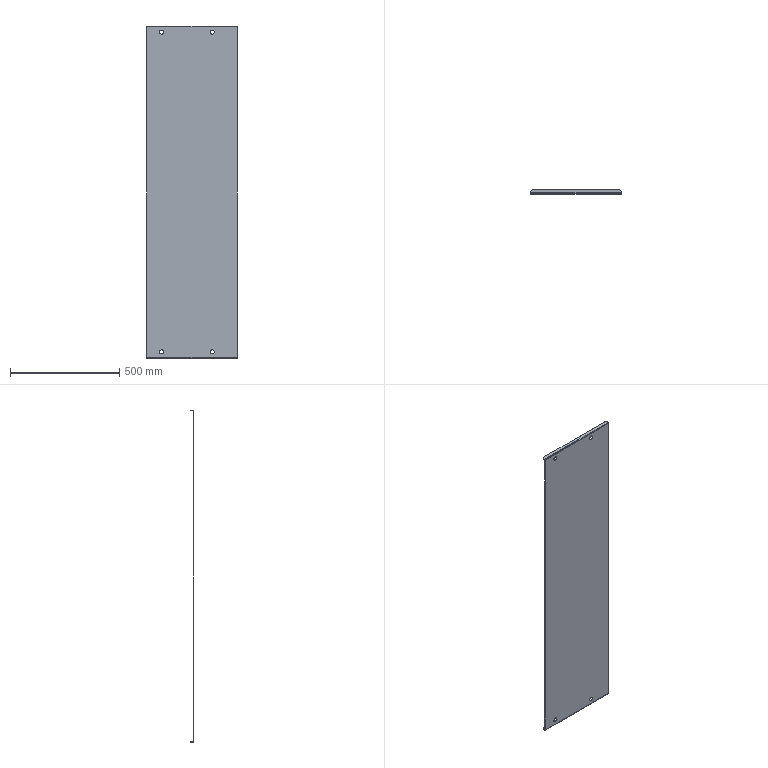Part | SolidWorks | features Fillet 1, FlatPattern 1, ICE 1, SMBaseFlange 1, SheetMetal 1 | 1 solid | 34 faces | box 413 x 18 x 1520 mm | volume 1023020 mm3 | plane 18 | cylinder 16 | commonest cylinder face diameters 18 x8 20 x4 3 x2 6.2 x2
STEP:
#1=CARTESIAN_POINT('',(-139.5,1.6,-1483.));
#2=VERTEX_POINT('',#1);
#3=CARTESIAN_POINT('',(-139.5,1.6,-1501.));
#4=VERTEX_POINT('',#3);
#5=CARTESIAN_POINT('',(-139.5,1.6,-1492.));
#6=DIRECTION('',(0.,-1.,0.));
#7=DIRECTION('',(0.,0.,1.));
#8=AXIS2_PLACEMENT_3D('',#5,#6,#7);
#9=CIRCLE('',#8,9.);
#10=EDGE_CURVE('',#2,#4,#9,.T.);
#11=ORIENTED_EDGE('',*,*,#10,.F.);
#12=CARTESIAN_POINT('',(-139.5,0.,-1483.));
#13=VERTEX_POINT('',#12);
#14=CARTESIAN_POINT('',(-139.5,18.001,-1483.));
#15=DIRECTION('',(0.,-1.,0.));
#16=VECTOR('',#15,1000.);
#17=LINE('',#14,#16);
#18=EDGE_CURVE('',#2,#13,#17,.T.);
#19=ORIENTED_EDGE('',*,*,#18,.T.);
#20=CARTESIAN_POINT('',(-139.5,0.,-1501.));
#21=VERTEX_POINT('',#20);
#22=CARTESIAN_POINT('',(-139.5,0.,-1492.));
#23=DIRECTION('',(0.,-1.,0.));
#24=DIRECTION('',(0.,0.,1.));
#25=AXIS2_PLACEMENT_3D('',#22,#23,#24);
#26=CIRCLE('',#25,9.);
#27=EDGE_CURVE('',#13,#21,#26,.T.);
#28=ORIENTED_EDGE('',*,*,#27,.T.);
#29=CARTESIAN_POINT('',(-139.5,18.001,-1501.));
#30=DIRECTION('',(0.,-1.,0.));
#31=VECTOR('',#30,1000.);
#32=LINE('',#29,#31);
#33=EDGE_CURVE('',#4,#21,#32,.T.);
#34=ORIENTED_EDGE('',*,*,#33,.F.);
#35=EDGE_LOOP('',(#11,#19,#28,#34));
#36=FACE_OUTER_BOUND('',#35,.T.);
#37=CARTESIAN_POINT('',(-139.5,18.001,-1492.));
#38=DIRECTION('',(0.,-1.,0.));
#39=DIRECTION('',(0.,0.,-1.));
#40=AXIS2_PLACEMENT_3D('',#37,#38,#39);
#41=CYLINDRICAL_SURFACE('',#40,9.);
#42=ADVANCED_FACE('',(#36),#41,.F.);
#43=CARTESIAN_POINT('',(92.5,1.6,-1483.));
#44=VERTEX_POINT('',#43);
#45=CARTESIAN_POINT('',(92.5,1.6,-1501.));
#46=VERTEX_POINT('',#45);
#47=CARTESIAN_POINT('',(92.5,1.6,-1492.));
#48=DIRECTION('',(0.,-1.,0.));
#49=DIRECTION('',(0.,0.,1.));
#50=AXIS2_PLACEMENT_3D('',#47,#48,#49);
#51=CIRCLE('',#50,9.);
#52=EDGE_CURVE('',#44,#46,#51,.T.);
#53=ORIENTED_EDGE('',*,*,#52,.F.);
#54=CARTESIAN_POINT('',(92.5,0.,-1483.));
#55=VERTEX_POINT('',#54);
#56=CARTESIAN_POINT('',(92.5,18.001,-1483.));
#57=DIRECTION('',(0.,-1.,0.));
#58=VECTOR('',#57,1000.);
#59=LINE('',#56,#58);
#60=EDGE_CURVE('',#44,#55,#59,.T.);
#61=ORIENTED_EDGE('',*,*,#60,.T.);
#62=CARTESIAN_POINT('',(92.5,0.,-1501.));
#63=VERTEX_POINT('',#62);
#64=CARTESIAN_POINT('',(92.5,0.,-1492.));
#65=DIRECTION('',(0.,-1.,0.));
#66=DIRECTION('',(0.,0.,1.));
#67=AXIS2_PLACEMENT_3D('',#64,#65,#66);
#68=CIRCLE('',#67,9.);
#69=EDGE_CURVE('',#55,#63,#68,.T.);
#70=ORIENTED_EDGE('',*,*,#69,.T.);
#71=CARTESIAN_POINT('',(92.5,18.001,-1501.));
#72=DIRECTION('',(0.,-1.,0.));
#73=VECTOR('',#72,1000.);
#74=LINE('',#71,#73);
#75=EDGE_CURVE('',#46,#63,#74,.T.);
#76=ORIENTED_EDGE('',*,*,#75,.F.);
#77=EDGE_LOOP('',(#53,#61,#70,#76));
#78=FACE_OUTER_BOUND('',#77,.T.);
#79=CARTESIAN_POINT('',(92.5,18.001,-1492.));
#80=DIRECTION('',(0.,-1.,0.));
#81=DIRECTION('',(0.,0.,-1.));
#82=AXIS2_PLACEMENT_3D('',#79,#80,#81);
#83=CYLINDRICAL_SURFACE('',#82,9.);
#84=ADVANCED_FACE('',(#78),#83,.F.);
#85=CARTESIAN_POINT('',(92.5,1.6,-19.));
#86=VERTEX_POINT('',#85);
#87=CARTESIAN_POINT('',(92.5,1.6,-37.));
#88=VERTEX_POINT('',#87);
#89=CARTESIAN_POINT('',(92.5,1.6,-28.));
#90=DIRECTION('',(0.,-1.,0.));
#91=DIRECTION('',(0.,0.,1.));
#92=AXIS2_PLACEMENT_3D('',#89,#90,#91);
#93=CIRCLE('',#92,9.);
#94=EDGE_CURVE('',#86,#88,#93,.T.);
#95=ORIENTED_EDGE('',*,*,#94,.F.);
#96=CARTESIAN_POINT('',(92.5,0.,-19.));
#97=VERTEX_POINT('',#96);
#98=CARTESIAN_POINT('',(92.5,18.001,-19.));
#99=DIRECTION('',(0.,-1.,0.));
#100=VECTOR('',#99,1000.);
#101=LINE('',#98,#100);
#102=EDGE_CURVE('',#86,#97,#101,.T.);
#103=ORIENTED_EDGE('',*,*,#102,.T.);
#104=CARTESIAN_POINT('',(92.5,0.,-37.));
#105=VERTEX_POINT('',#104);
#106=CARTESIAN_POINT('',(92.5,0.,-28.));
#107=DIRECTION('',(0.,-1.,0.));
#108=DIRECTION('',(0.,0.,-1.));
#109=AXIS2_PLACEMENT_3D('',#106,#107,#108);
#110=CIRCLE('',#109,9.);
#111=EDGE_CURVE('',#97,#105,#110,.T.);
#112=ORIENTED_EDGE('',*,*,#111,.T.);
#113=CARTESIAN_POINT('',(92.5,18.001,-37.));
#114=DIRECTION('',(0.,-1.,0.));
#115=VECTOR('',#114,1000.);
#116=LINE('',#113,#115);
#117=EDGE_CURVE('',#88,#105,#116,.T.);
#118=ORIENTED_EDGE('',*,*,#117,.F.);
#119=EDGE_LOOP('',(#95,#103,#112,#118));
#120=FACE_OUTER_BOUND('',#119,.T.);
#121=CARTESIAN_POINT('',(92.5,18.001,-28.));
#122=DIRECTION('',(0.,-1.,0.));
#123=DIRECTION('',(0.,0.,-1.));
#124=AXIS2_PLACEMENT_3D('',#121,#122,#123);
#125=CYLINDRICAL_SURFACE('',#124,9.);
#126=ADVANCED_FACE('',(#120),#125,.F.);
#127=CARTESIAN_POINT('',(-139.5,1.6,-19.));
#128=VERTEX_POINT('',#127);
#129=CARTESIAN_POINT('',(-139.5,1.6,-37.));
#130=VERTEX_POINT('',#129);
#131=CARTESIAN_POINT('',(-139.5,1.6,-28.));
#132=DIRECTION('',(0.,-1.,0.));
#133=DIRECTION('',(0.,0.,1.));
#134=AXIS2_PLACEMENT_3D('',#131,#132,#133);
#135=CIRCLE('',#134,9.);
#136=EDGE_CURVE('',#128,#130,#135,.T.);
#137=ORIENTED_EDGE('',*,*,#136,.F.);
#138=CARTESIAN_POINT('',(-139.5,0.,-19.));
#139=VERTEX_POINT('',#138);
#140=CARTESIAN_POINT('',(-139.5,18.001,-19.));
#141=DIRECTION('',(0.,-1.,0.));
#142=VECTOR('',#141,1000.);
#143=LINE('',#140,#142);
#144=EDGE_CURVE('',#128,#139,#143,.T.);
#145=ORIENTED_EDGE('',*,*,#144,.T.);
#146=CARTESIAN_POINT('',(-139.5,0.,-37.));
#147=VERTEX_POINT('',#146);
#148=CARTESIAN_POINT('',(-139.5,0.,-28.));
#149=DIRECTION('',(0.,-1.,0.));
#150=DIRECTION('',(0.,0.,-1.));
#151=AXIS2_PLACEMENT_3D('',#148,#149,#150);
#152=CIRCLE('',#151,9.);
#153=EDGE_CURVE('',#139,#147,#152,.T.);
#154=ORIENTED_EDGE('',*,*,#153,.T.);
#155=CARTESIAN_POINT('',(-139.5,18.001,-37.));
#156=DIRECTION('',(0.,-1.,0.));
#157=VECTOR('',#156,1000.);
#158=LINE('',#155,#157);
#159=EDGE_CURVE('',#130,#147,#158,.T.);
#160=ORIENTED_EDGE('',*,*,#159,.F.);
#161=EDGE_LOOP('',(#137,#145,#154,#160));
#162=FACE_OUTER_BOUND('',#161,.T.);
#163=CARTESIAN_POINT('',(-139.5,18.001,-28.));
#164=DIRECTION('',(0.,-1.,0.));
#165=DIRECTION('',(0.,0.,-1.));
#166=AXIS2_PLACEMENT_3D('',#163,#164,#165);
#167=CYLINDRICAL_SURFACE('',#166,9.);
#168=ADVANCED_FACE('',(#162),#167,.F.);
#169=CARTESIAN_POINT('',(206.5,3.1,0.));
#170=VERTEX_POINT('',#169);
#171=CARTESIAN_POINT('',(206.5,3.1,-1.6));
#172=VERTEX_POINT('',#171);
#173=CARTESIAN_POINT('',(206.5,3.1,0.));
#174=DIRECTION('',(0.,0.,-1.));
#175=VECTOR('',#174,1000.);
#176=LINE('',#173,#175);
#177=EDGE_CURVE('',#170,#172,#176,.T.);
#178=ORIENTED_EDGE('',*,*,#177,.F.);
#179=CARTESIAN_POINT('',(206.5,0.,-3.1));
#180=VERTEX_POINT('',#179);
#181=CARTESIAN_POINT('',(206.5,3.1,-3.1));
#182=DIRECTION('',(1.,0.,0.));
#183=DIRECTION('',(0.,0.,1.));
#184=AXIS2_PLACEMENT_3D('',#181,#182,#183);
#185=CIRCLE('',#184,3.1);
#186=EDGE_CURVE('',#170,#180,#185,.T.);
#187=ORIENTED_EDGE('',*,*,#186,.T.);
#188=CARTESIAN_POINT('',(206.5,1.6,-3.1));
#189=VERTEX_POINT('',#188);
#190=CARTESIAN_POINT('',(206.5,1.6,-3.1));
#191=DIRECTION('',(0.,-1.,0.));
#192=VECTOR('',#191,1000.);
#193=LINE('',#190,#192);
#194=EDGE_CURVE('',#189,#180,#193,.T.);
#195=ORIENTED_EDGE('',*,*,#194,.F.);
#196=CARTESIAN_POINT('',(206.5,3.1,-3.1));
#197=DIRECTION('',(1.,0.,0.));
#198=DIRECTION('',(0.,0.,-1.));
#199=AXIS2_PLACEMENT_3D('',#196,#197,#198);
#200=CIRCLE('',#199,1.5);
#201=EDGE_CURVE('',#172,#189,#200,.T.);
#202=ORIENTED_EDGE('',*,*,#201,.F.);
#203=EDGE_LOOP('',(#178,#187,#195,#202));
#204=FACE_OUTER_BOUND('',#203,.T.);
#205=CARTESIAN_POINT('',(206.5,3.1,0.));
#206=DIRECTION('',(1.,0.,0.));
#207=DIRECTION('',(0.,0.,-1.));
#208=AXIS2_PLACEMENT_3D('',#205,#206,#207);
#209=PLANE('',#208);
#210=ADVANCED_FACE('',(#204),#209,.T.);
#211=CARTESIAN_POINT('',(206.5,8.,-1.6));
#212=VERTEX_POINT('',#211);
#213=CARTESIAN_POINT('',(206.5,0.,-1.6));
#214=DIRECTION('',(0.,-1.,0.));
#215=VECTOR('',#214,1000.);
#216=LINE('',#213,#215);
#217=EDGE_CURVE('',#212,#172,#216,.T.);
#218=ORIENTED_EDGE('',*,*,#217,.F.);
#219=CARTESIAN_POINT('',(206.5,8.,0.));
#220=VERTEX_POINT('',#219);
#221=CARTESIAN_POINT('',(206.5,8.,-3.1));
#222=DIRECTION('',(0.,0.,1.));
#223=VECTOR('',#222,1000.);
#224=LINE('',#221,#223);
#225=EDGE_CURVE('',#212,#220,#224,.T.);
#226=ORIENTED_EDGE('',*,*,#225,.T.);
#227=CARTESIAN_POINT('',(206.5,0.,0.));
#228=DIRECTION('',(0.,-1.,0.));
#229=VECTOR('',#228,1000.);
#230=LINE('',#227,#229);
#231=EDGE_CURVE('',#220,#170,#230,.T.);
#232=ORIENTED_EDGE('',*,*,#231,.T.);
#233=ORIENTED_EDGE('',*,*,#177,.T.);
#234=EDGE_LOOP('',(#218,#226,#232,#233));
#235=FACE_OUTER_BOUND('',#234,.T.);
#236=CARTESIAN_POINT('',(206.5,1.6,-3.1));
#237=DIRECTION('',(1.,0.,0.));
#238=DIRECTION('',(0.,0.,-1.));
#239=AXIS2_PLACEMENT_3D('',#236,#237,#238);
#240=PLANE('',#239);
#241=ADVANCED_FACE('',(#235),#240,.T.);
#242=CARTESIAN_POINT('',(-206.5,0.,-3.1));
#243=VERTEX_POINT('',#242);
#244=CARTESIAN_POINT('',(-206.5,1.6,-3.1));
#245=VERTEX_POINT('',#244);
#246=CARTESIAN_POINT('',(-206.5,0.,-3.1));
#247=DIRECTION('',(0.,1.,0.));
#248=VECTOR('',#247,1000.);
#249=LINE('',#246,#248);
#250=EDGE_CURVE('',#243,#245,#249,.T.);
#251=ORIENTED_EDGE('',*,*,#250,.F.);
#252=CARTESIAN_POINT('',(-206.5,3.1,0.));
#253=VERTEX_POINT('',#252);
#254=CARTESIAN_POINT('',(-206.5,3.1,-3.1));
#255=DIRECTION('',(1.,0.,0.));
#256=DIRECTION('',(0.,0.,1.));
#257=AXIS2_PLACEMENT_3D('',#254,#255,#256);
#258=CIRCLE('',#257,3.1);
#259=EDGE_CURVE('',#253,#243,#258,.T.);
#260=ORIENTED_EDGE('',*,*,#259,.F.);
#261=CARTESIAN_POINT('',(-206.5,3.1,-1.6));
#262=VERTEX_POINT('',#261);
#263=CARTESIAN_POINT('',(-206.5,3.1,-1.6));
#264=DIRECTION('',(0.,0.,1.));
#265=VECTOR('',#264,1000.);
#266=LINE('',#263,#265);
#267=EDGE_CURVE('',#262,#253,#266,.T.);
#268=ORIENTED_EDGE('',*,*,#267,.F.);
#269=CARTESIAN_POINT('',(-206.5,3.1,-3.1));
#270=DIRECTION('',(1.,0.,0.));
#271=DIRECTION('',(0.,0.,-1.));
#272=AXIS2_PLACEMENT_3D('',#269,#270,#271);
#273=CIRCLE('',#272,1.5);
#274=EDGE_CURVE('',#262,#245,#273,.T.);
#275=ORIENTED_EDGE('',*,*,#274,.T.);
#276=EDGE_LOOP('',(#251,#260,#268,#275));
#277=FACE_OUTER_BOUND('',#276,.T.);
#278=CARTESIAN_POINT('',(-206.5,0.,-3.1));
#279=DIRECTION('',(-1.,0.,0.));
#280=DIRECTION('',(0.,0.,1.));
#281=AXIS2_PLACEMENT_3D('',#278,#279,#280);
#282=PLANE('',#281);
#283=ADVANCED_FACE('',(#277),#282,.T.);
#284=CARTESIAN_POINT('',(-206.5,0.,-1516.9));
#285=VERTEX_POINT('',#284);
#286=CARTESIAN_POINT('',(-206.5,0.,0.));
#287=DIRECTION('',(0.,0.,-1.));
#288=VECTOR('',#287,1000.);
#289=LINE('',#286,#288);
#290=EDGE_CURVE('',#243,#285,#289,.T.);
#291=ORIENTED_EDGE('',*,*,#290,.F.);
#292=ORIENTED_EDGE('',*,*,#250,.T.);
#293=CARTESIAN_POINT('',(-206.5,1.6,-1516.9));
#294=VERTEX_POINT('',#293);
#295=CARTESIAN_POINT('',(-206.5,1.6,0.));
#296=DIRECTION('',(0.,0.,-1.));
#297=VECTOR('',#296,1000.);
#298=LINE('',#295,#297);
#299=EDGE_CURVE('',#245,#294,#298,.T.);
#300=ORIENTED_EDGE('',*,*,#299,.T.);
#301=CARTESIAN_POINT('',(-206.5,1.6,-1516.9));
#302=DIRECTION('',(0.,-1.,0.));
#303=VECTOR('',#302,1000.);
#304=LINE('',#301,#303);
#305=EDGE_CURVE('',#294,#285,#304,.T.);
#306=ORIENTED_EDGE('',*,*,#305,.T.);
#307=EDGE_LOOP('',(#291,#292,#300,#306));
#308=FACE_OUTER_BOUND('',#307,.T.);
#309=CARTESIAN_POINT('',(-206.5,3.1,-1.6));
#310=DIRECTION('',(-1.,0.,0.));
#311=DIRECTION('',(0.,0.,1.));
#312=AXIS2_PLACEMENT_3D('',#309,#310,#311);
#313=PLANE('',#312);
#314=ADVANCED_FACE('',(#308),#313,.T.);
#315=CARTESIAN_POINT('',(206.5,0.,-1516.9));
#316=VERTEX_POINT('',#315);
#317=CARTESIAN_POINT('',(206.5,1.6,-1516.9));
#318=VERTEX_POINT('',#317);
#319=CARTESIAN_POINT('',(206.5,0.,-1516.9));
#320=DIRECTION('',(0.,1.,0.));
#321=VECTOR('',#320,1000.);
#322=LINE('',#319,#321);
#323=EDGE_CURVE('',#316,#318,#322,.T.);
#324=ORIENTED_EDGE('',*,*,#323,.F.);
#325=CARTESIAN_POINT('',(206.5,3.1,-1520.));
#326=VERTEX_POINT('',#325);
#327=CARTESIAN_POINT('',(206.5,3.1,-1516.9));
#328=DIRECTION('',(1.,0.,0.));
#329=DIRECTION('',(0.,0.,1.));
#330=AXIS2_PLACEMENT_3D('',#327,#328,#329);
#331=CIRCLE('',#330,3.1);
#332=EDGE_CURVE('',#316,#326,#331,.T.);
#333=ORIENTED_EDGE('',*,*,#332,.T.);
#334=CARTESIAN_POINT('',(206.5,3.1,-1518.4));
#335=VERTEX_POINT('',#334);
#336=CARTESIAN_POINT('',(206.5,3.1,-1518.4));
#337=DIRECTION('',(0.,0.,-1.));
#338=VECTOR('',#337,1000.);
#339=LINE('',#336,#338);
#340=EDGE_CURVE('',#335,#326,#339,.T.);
#341=ORIENTED_EDGE('',*,*,#340,.F.);
#342=CARTESIAN_POINT('',(206.5,3.1,-1516.9));
#343=DIRECTION('',(1.,0.,0.));
#344=DIRECTION('',(0.,0.,-1.));
#345=AXIS2_PLACEMENT_3D('',#342,#343,#344);
#346=CIRCLE('',#345,1.5);
#347=EDGE_CURVE('',#318,#335,#346,.T.);
#348=ORIENTED_EDGE('',*,*,#347,.F.);
#349=EDGE_LOOP('',(#324,#333,#341,#348));
#350=FACE_OUTER_BOUND('',#349,.T.);
#351=CARTESIAN_POINT('',(206.5,0.,-1516.9));
#352=DIRECTION('',(1.,0.,0.));
#353=DIRECTION('',(0.,0.,-1.));
#354=AXIS2_PLACEMENT_3D('',#351,#352,#353);
#355=PLANE('',#354);
#356=ADVANCED_FACE('',(#350),#355,.T.);
#357=CARTESIAN_POINT('',(206.5,0.,0.));
#358=DIRECTION('',(0.,0.,-1.));
#359=VECTOR('',#358,1000.);
#360=LINE('',#357,#359);
#361=EDGE_CURVE('',#180,#316,#360,.T.);
#362=ORIENTED_EDGE('',*,*,#361,.T.);
#363=ORIENTED_EDGE('',*,*,#323,.T.);
#364=CARTESIAN_POINT('',(206.5,1.6,0.));
#365=DIRECTION('',(0.,0.,-1.));
#366=VECTOR('',#365,1000.);
#367=LINE('',#364,#366);
#368=EDGE_CURVE('',#189,#318,#367,.T.);
#369=ORIENTED_EDGE('',*,*,#368,.F.);
#370=ORIENTED_EDGE('',*,*,#194,.T.);
#371=EDGE_LOOP('',(#362,#363,#369,#370));
#372=FACE_OUTER_BOUND('',#371,.T.);
#373=CARTESIAN_POINT('',(206.5,3.1,-1518.4));
#374=DIRECTION('',(1.,0.,0.));
#375=DIRECTION('',(0.,0.,-1.));
#376=AXIS2_PLACEMENT_3D('',#373,#374,#375);
#377=PLANE('',#376);
#378=ADVANCED_FACE('',(#372),#377,.T.);
#379=CARTESIAN_POINT('',(-206.5,3.1,-1520.));
#380=VERTEX_POINT('',#379);
#381=CARTESIAN_POINT('',(-206.5,3.1,-1518.4));
#382=VERTEX_POINT('',#381);
#383=CARTESIAN_POINT('',(-206.5,3.1,-1520.));
#384=DIRECTION('',(0.,0.,1.));
#385=VECTOR('',#384,1000.);
#386=LINE('',#383,#385);
#387=EDGE_CURVE('',#380,#382,#386,.T.);
#388=ORIENTED_EDGE('',*,*,#387,.F.);
#389=CARTESIAN_POINT('',(-206.5,3.1,-1516.9));
#390=DIRECTION('',(1.,0.,0.));
#391=DIRECTION('',(0.,0.,1.));
#392=AXIS2_PLACEMENT_3D('',#389,#390,#391);
#393=CIRCLE('',#392,3.1);
#394=EDGE_CURVE('',#285,#380,#393,.T.);
#395=ORIENTED_EDGE('',*,*,#394,.F.);
#396=ORIENTED_EDGE('',*,*,#305,.F.);
#397=CARTESIAN_POINT('',(-206.5,3.1,-1516.9));
#398=DIRECTION('',(1.,0.,0.));
#399=DIRECTION('',(0.,0.,-1.));
#400=AXIS2_PLACEMENT_3D('',#397,#398,#399);
#401=CIRCLE('',#400,1.5);
#402=EDGE_CURVE('',#294,#382,#401,.T.);
#403=ORIENTED_EDGE('',*,*,#402,.T.);
#404=EDGE_LOOP('',(#388,#395,#396,#403));
#405=FACE_OUTER_BOUND('',#404,.T.);
#406=CARTESIAN_POINT('',(-206.5,3.1,-1520.));
#407=DIRECTION('',(-1.,0.,0.));
#408=DIRECTION('',(0.,0.,1.));
#409=AXIS2_PLACEMENT_3D('',#406,#407,#408);
#410=PLANE('',#409);
#411=ADVANCED_FACE('',(#405),#410,.T.);
#412=CARTESIAN_POINT('',(-206.5,8.,-1518.4));
#413=VERTEX_POINT('',#412);
#414=CARTESIAN_POINT('',(-206.5,0.,-1518.4));
#415=DIRECTION('',(0.,1.,0.));
#416=VECTOR('',#415,1000.);
#417=LINE('',#414,#416);
#418=EDGE_CURVE('',#382,#413,#417,.T.);
#419=ORIENTED_EDGE('',*,*,#418,.T.);
#420=CARTESIAN_POINT('',(-206.5,8.,-1520.));
#421=VERTEX_POINT('',#420);
#422=CARTESIAN_POINT('',(-206.5,8.,-1516.9));
#423=DIRECTION('',(0.,0.,-1.));
#424=VECTOR('',#423,1000.);
#425=LINE('',#422,#424);
#426=EDGE_CURVE('',#413,#421,#425,.T.);
#427=ORIENTED_EDGE('',*,*,#426,.T.);
#428=CARTESIAN_POINT('',(-206.5,0.,-1520.));
#429=DIRECTION('',(0.,1.,0.));
#430=VECTOR('',#429,1000.);
#431=LINE('',#428,#430);
#432=EDGE_CURVE('',#380,#421,#431,.T.);
#433=ORIENTED_EDGE('',*,*,#432,.F.);
#434=ORIENTED_EDGE('',*,*,#387,.T.);
#435=EDGE_LOOP('',(#419,#427,#433,#434));
#436=FACE_OUTER_BOUND('',#435,.T.);
#437=CARTESIAN_POINT('',(-206.5,1.6,-1516.9));
#438=DIRECTION('',(-1.,0.,0.));
#439=DIRECTION('',(0.,0.,1.));
#440=AXIS2_PLACEMENT_3D('',#437,#438,#439);
#441=PLANE('',#440);
#442=ADVANCED_FACE('',(#436),#441,.T.);
#443=ORIENTED_EDGE('',*,*,#432,.T.);
#444=CARTESIAN_POINT('',(-196.5,18.,-1520.));
#445=VERTEX_POINT('',#444);
#446=CARTESIAN_POINT('',(-196.5,8.,-1520.));
#447=DIRECTION('',(0.,0.,-1.));
#448=DIRECTION('',(1.,0.,0.));
#449=AXIS2_PLACEMENT_3D('',#446,#447,#448);
#450=CIRCLE('',#449,10.);
#451=EDGE_CURVE('',#421,#445,#450,.T.);
#452=ORIENTED_EDGE('',*,*,#451,.T.);
#453=CARTESIAN_POINT('',(196.5,18.,-1520.));
#454=VERTEX_POINT('',#453);
#455=CARTESIAN_POINT('',(206.5,18.,-1520.));
#456=DIRECTION('',(-1.,0.,0.));
#457=VECTOR('',#456,1000.);
#458=LINE('',#455,#457);
#459=EDGE_CURVE('',#454,#445,#458,.T.);
#460=ORIENTED_EDGE('',*,*,#459,.F.);
#461=CARTESIAN_POINT('',(206.5,8.,-1520.));
#462=VERTEX_POINT('',#461);
#463=CARTESIAN_POINT('',(196.5,8.,-1520.));
#464=DIRECTION('',(0.,0.,-1.));
#465=DIRECTION('',(1.,0.,0.));
#466=AXIS2_PLACEMENT_3D('',#463,#464,#465);
#467=CIRCLE('',#466,10.);
#468=EDGE_CURVE('',#454,#462,#467,.T.);
#469=ORIENTED_EDGE('',*,*,#468,.T.);
#470=CARTESIAN_POINT('',(206.5,0.,-1520.));
#471=DIRECTION('',(0.,1.,0.));
#472=VECTOR('',#471,1000.);
#473=LINE('',#470,#472);
#474=EDGE_CURVE('',#326,#462,#473,.T.);
#475=ORIENTED_EDGE('',*,*,#474,.F.);
#476=CARTESIAN_POINT('',(206.5,3.1,-1520.));
#477=DIRECTION('',(-1.,0.,0.));
#478=VECTOR('',#477,1000.);
#479=LINE('',#476,#478);
#480=EDGE_CURVE('',#326,#380,#479,.T.);
#481=ORIENTED_EDGE('',*,*,#480,.T.);
#482=EDGE_LOOP('',(#443,#452,#460,#469,#475,#481));
#483=FACE_OUTER_BOUND('',#482,.T.);
#484=CARTESIAN_POINT('',(206.5,0.,-1520.));
#485=DIRECTION('',(0.,0.,1.));
#486=DIRECTION('',(1.,0.,0.));
#487=AXIS2_PLACEMENT_3D('',#484,#485,#486);
#488=PLANE('',#487);
#489=ADVANCED_FACE('',(#483),#488,.F.);
#490=ORIENTED_EDGE('',*,*,#459,.T.);
#491=CARTESIAN_POINT('',(-196.5,18.,-1518.4));
#492=VERTEX_POINT('',#491);
#493=CARTESIAN_POINT('',(-196.5,18.,-1518.4));
#494=DIRECTION('',(0.,0.,1.));
#495=VECTOR('',#494,1000.);
#496=LINE('',#493,#495);
#497=EDGE_CURVE('',#445,#492,#496,.T.);
#498=ORIENTED_EDGE('',*,*,#497,.T.);
#499=CARTESIAN_POINT('',(196.5,18.,-1518.4));
#500=VERTEX_POINT('',#499);
#501=CARTESIAN_POINT('',(206.5,18.,-1518.4));
#502=DIRECTION('',(-1.,0.,0.));
#503=VECTOR('',#502,1000.);
#504=LINE('',#501,#503);
#505=EDGE_CURVE('',#500,#492,#504,.T.);
#506=ORIENTED_EDGE('',*,*,#505,.F.);
#507=CARTESIAN_POINT('',(196.5,18.,-1518.4));
#508=DIRECTION('',(0.,0.,-1.));
#509=VECTOR('',#508,1000.);
#510=LINE('',#507,#509);
#511=EDGE_CURVE('',#500,#454,#510,.T.);
#512=ORIENTED_EDGE('',*,*,#511,.T.);
#513=EDGE_LOOP('',(#490,#498,#506,#512));
#514=FACE_OUTER_BOUND('',#513,.T.);
#515=CARTESIAN_POINT('',(206.5,18.,-1518.4));
#516=DIRECTION('',(0.,1.,0.));
#517=DIRECTION('',(0.,0.,1.));
#518=AXIS2_PLACEMENT_3D('',#515,#516,#517);
#519=PLANE('',#518);
#520=ADVANCED_FACE('',(#514),#519,.T.);
#521=ORIENTED_EDGE('',*,*,#505,.T.);
#522=CARTESIAN_POINT('',(-196.5,8.,-1518.4));
#523=DIRECTION('',(0.,0.,1.));
#524=DIRECTION('',(1.,0.,0.));
#525=AXIS2_PLACEMENT_3D('',#522,#523,#524);
#526=CIRCLE('',#525,10.);
#527=EDGE_CURVE('',#492,#413,#526,.T.);
#528=ORIENTED_EDGE('',*,*,#527,.T.);
#529=ORIENTED_EDGE('',*,*,#418,.F.);
#530=CARTESIAN_POINT('',(206.5,3.1,-1518.4));
#531=DIRECTION('',(-1.,0.,0.));
#532=VECTOR('',#531,1000.);
#533=LINE('',#530,#532);
#534=EDGE_CURVE('',#335,#382,#533,.T.);
#535=ORIENTED_EDGE('',*,*,#534,.F.);
#536=CARTESIAN_POINT('',(206.5,8.,-1518.4));
#537=VERTEX_POINT('',#536);
#538=CARTESIAN_POINT('',(206.5,0.,-1518.4));
#539=DIRECTION('',(0.,1.,0.));
#540=VECTOR('',#539,1000.);
#541=LINE('',#538,#540);
#542=EDGE_CURVE('',#335,#537,#541,.T.);
#543=ORIENTED_EDGE('',*,*,#542,.T.);
#544=CARTESIAN_POINT('',(196.5,8.,-1518.4));
#545=DIRECTION('',(0.,0.,1.));
#546=DIRECTION('',(1.,0.,0.));
#547=AXIS2_PLACEMENT_3D('',#544,#545,#546);
#548=CIRCLE('',#547,10.);
#549=EDGE_CURVE('',#537,#500,#548,.T.);
#550=ORIENTED_EDGE('',*,*,#549,.T.);
#551=EDGE_LOOP('',(#521,#528,#529,#535,#543,#550));
#552=FACE_OUTER_BOUND('',#551,.T.);
#553=CARTESIAN_POINT('',(206.5,0.,-1518.4));
#554=DIRECTION('',(0.,0.,1.));
#555=DIRECTION('',(1.,0.,0.));
#556=AXIS2_PLACEMENT_3D('',#553,#554,#555);
#557=PLANE('',#556);
#558=ADVANCED_FACE('',(#552),#557,.T.);
#559=ORIENTED_EDGE('',*,*,#402,.F.);
#560=CARTESIAN_POINT('',(206.5,1.6,-1516.9));
#561=DIRECTION('',(-1.,0.,0.));
#562=VECTOR('',#561,1000.);
#563=LINE('',#560,#562);
#564=EDGE_CURVE('',#318,#294,#563,.T.);
#565=ORIENTED_EDGE('',*,*,#564,.F.);
#566=ORIENTED_EDGE('',*,*,#347,.T.);
#567=ORIENTED_EDGE('',*,*,#534,.T.);
#568=EDGE_LOOP('',(#559,#565,#566,#567));
#569=FACE_OUTER_BOUND('',#568,.T.);
#570=CARTESIAN_POINT('',(206.5,3.1,-1516.9));
#571=DIRECTION('',(-1.,0.,0.));
#572=DIRECTION('',(0.,0.,1.));
#573=AXIS2_PLACEMENT_3D('',#570,#571,#572);
#574=CYLINDRICAL_SURFACE('',#573,1.5);
#575=ADVANCED_FACE('',(#569),#574,.F.);
#576=CARTESIAN_POINT('',(-139.5,1.6,-1492.));
#577=DIRECTION('',(0.,-1.,0.));
#578=DIRECTION('',(0.,0.,1.));
#579=AXIS2_PLACEMENT_3D('',#576,#577,#578);
#580=CIRCLE('',#579,9.);
#581=EDGE_CURVE('',#4,#2,#580,.T.);
#582=ORIENTED_EDGE('',*,*,#581,.T.);
#583=ORIENTED_EDGE('',*,*,#10,.T.);
#584=EDGE_LOOP('',(#582,#583));
#585=FACE_BOUND('',#584,.T.);
#586=CARTESIAN_POINT('',(92.5,1.6,-1492.));
#587=DIRECTION('',(0.,-1.,0.));
#588=DIRECTION('',(0.,0.,1.));
#589=AXIS2_PLACEMENT_3D('',#586,#587,#588);
#590=CIRCLE('',#589,9.);
#591=EDGE_CURVE('',#46,#44,#590,.T.);
#592=ORIENTED_EDGE('',*,*,#591,.T.);
#593=ORIENTED_EDGE('',*,*,#52,.T.);
#594=EDGE_LOOP('',(#592,#593));
#595=FACE_BOUND('',#594,.T.);
#596=CARTESIAN_POINT('',(92.5,1.6,-28.));
#597=DIRECTION('',(0.,-1.,0.));
#598=DIRECTION('',(0.,0.,1.));
#599=AXIS2_PLACEMENT_3D('',#596,#597,#598);
#600=CIRCLE('',#599,9.);
#601=EDGE_CURVE('',#88,#86,#600,.T.);
#602=ORIENTED_EDGE('',*,*,#601,.T.);
#603=ORIENTED_EDGE('',*,*,#94,.T.);
#604=EDGE_LOOP('',(#602,#603));
#605=FACE_BOUND('',#604,.T.);
#606=CARTESIAN_POINT('',(-139.5,1.6,-28.));
#607=DIRECTION('',(0.,-1.,0.));
#608=DIRECTION('',(0.,0.,1.));
#609=AXIS2_PLACEMENT_3D('',#606,#607,#608);
#610=CIRCLE('',#609,9.);
#611=EDGE_CURVE('',#130,#128,#610,.T.);
#612=ORIENTED_EDGE('',*,*,#611,.T.);
#613=ORIENTED_EDGE('',*,*,#136,.T.);
#614=EDGE_LOOP('',(#612,#613));
#615=FACE_BOUND('',#614,.T.);
#616=ORIENTED_EDGE('',*,*,#299,.F.);
#617=CARTESIAN_POINT('',(206.5,1.6,-3.1));
#618=DIRECTION('',(-1.,0.,0.));
#619=VECTOR('',#618,1000.);
#620=LINE('',#617,#619);
#621=EDGE_CURVE('',#189,#245,#620,.T.);
#622=ORIENTED_EDGE('',*,*,#621,.F.);
#623=ORIENTED_EDGE('',*,*,#368,.T.);
#624=ORIENTED_EDGE('',*,*,#564,.T.);
#625=EDGE_LOOP('',(#616,#622,#623,#624));
#626=FACE_OUTER_BOUND('',#625,.T.);
#627=CARTESIAN_POINT('',(206.5,1.6,0.));
#628=DIRECTION('',(0.,1.,0.));
#629=DIRECTION('',(0.,0.,1.));
#630=AXIS2_PLACEMENT_3D('',#627,#628,#629);
#631=PLANE('',#630);
#632=ADVANCED_FACE('',(#585,#595,#605,#615,#626),#631,.T.);
#633=ORIENTED_EDGE('',*,*,#274,.F.);
#634=CARTESIAN_POINT('',(206.5,3.1,-1.6));
#635=DIRECTION('',(-1.,0.,0.));
#636=VECTOR('',#635,1000.);
#637=LINE('',#634,#636);
#638=EDGE_CURVE('',#172,#262,#637,.T.);
#639=ORIENTED_EDGE('',*,*,#638,.F.);
#640=ORIENTED_EDGE('',*,*,#201,.T.);
#641=ORIENTED_EDGE('',*,*,#621,.T.);
#642=EDGE_LOOP('',(#633,#639,#640,#641));
#643=FACE_OUTER_BOUND('',#642,.T.);
#644=CARTESIAN_POINT('',(206.5,3.1,-3.1));
#645=DIRECTION('',(-1.,0.,0.));
#646=DIRECTION('',(0.,0.,1.));
#647=AXIS2_PLACEMENT_3D('',#644,#645,#646);
#648=CYLINDRICAL_SURFACE('',#647,1.5);
#649=ADVANCED_FACE('',(#643),#648,.F.);
#650=CARTESIAN_POINT('',(196.5,18.,-1.6));
#651=VERTEX_POINT('',#650);
#652=CARTESIAN_POINT('',(-196.5,18.,-1.6));
#653=VERTEX_POINT('',#652);
#654=CARTESIAN_POINT('',(206.5,18.,-1.6));
#655=DIRECTION('',(-1.,0.,0.));
#656=VECTOR('',#655,1000.);
#657=LINE('',#654,#656);
#658=EDGE_CURVE('',#651,#653,#657,.T.);
#659=ORIENTED_EDGE('',*,*,#658,.F.);
#660=CARTESIAN_POINT('',(196.5,8.,-1.6));
#661=DIRECTION('',(0.,0.,-1.));
#662=DIRECTION('',(-1.,0.,0.));
#663=AXIS2_PLACEMENT_3D('',#660,#661,#662);
#664=CIRCLE('',#663,10.);
#665=EDGE_CURVE('',#651,#212,#664,.T.);
#666=ORIENTED_EDGE('',*,*,#665,.T.);
#667=ORIENTED_EDGE('',*,*,#217,.T.);
#668=ORIENTED_EDGE('',*,*,#638,.T.);
#669=CARTESIAN_POINT('',(-206.5,8.,-1.6));
#670=VERTEX_POINT('',#669);
#671=CARTESIAN_POINT('',(-206.5,0.,-1.6));
#672=DIRECTION('',(0.,-1.,0.));
#673=VECTOR('',#672,1000.);
#674=LINE('',#671,#673);
#675=EDGE_CURVE('',#670,#262,#674,.T.);
#676=ORIENTED_EDGE('',*,*,#675,.F.);
#677=CARTESIAN_POINT('',(-196.5,8.,-1.6));
#678=DIRECTION('',(0.,0.,-1.));
#679=DIRECTION('',(-1.,0.,0.));
#680=AXIS2_PLACEMENT_3D('',#677,#678,#679);
#681=CIRCLE('',#680,10.);
#682=EDGE_CURVE('',#670,#653,#681,.T.);
#683=ORIENTED_EDGE('',*,*,#682,.T.);
#684=EDGE_LOOP('',(#659,#666,#667,#668,#676,#683));
#685=FACE_OUTER_BOUND('',#684,.T.);
#686=CARTESIAN_POINT('',(206.5,0.,-1.6));
#687=DIRECTION('',(0.,0.,-1.));
#688=DIRECTION('',(-1.,0.,0.));
#689=AXIS2_PLACEMENT_3D('',#686,#687,#688);
#690=PLANE('',#689);
#691=ADVANCED_FACE('',(#685),#690,.T.);
#692=CARTESIAN_POINT('',(196.5,18.,0.));
#693=VERTEX_POINT('',#692);
#694=CARTESIAN_POINT('',(-196.5,18.,0.));
#695=VERTEX_POINT('',#694);
#696=CARTESIAN_POINT('',(206.5,18.,0.));
#697=DIRECTION('',(-1.,0.,0.));
#698=VECTOR('',#697,1000.);
#699=LINE('',#696,#698);
#700=EDGE_CURVE('',#693,#695,#699,.T.);
#701=ORIENTED_EDGE('',*,*,#700,.F.);
#702=CARTESIAN_POINT('',(196.5,18.,0.));
#703=DIRECTION('',(0.,0.,-1.));
#704=VECTOR('',#703,1000.);
#705=LINE('',#702,#704);
#706=EDGE_CURVE('',#693,#651,#705,.T.);
#707=ORIENTED_EDGE('',*,*,#706,.T.);
#708=ORIENTED_EDGE('',*,*,#658,.T.);
#709=CARTESIAN_POINT('',(-196.5,18.,0.));
#710=DIRECTION('',(0.,0.,1.));
#711=VECTOR('',#710,1000.);
#712=LINE('',#709,#711);
#713=EDGE_CURVE('',#653,#695,#712,.T.);
#714=ORIENTED_EDGE('',*,*,#713,.T.);
#715=EDGE_LOOP('',(#701,#707,#708,#714));
#716=FACE_OUTER_BOUND('',#715,.T.);
#717=CARTESIAN_POINT('',(206.5,18.,0.));
#718=DIRECTION('',(0.,1.,0.));
#719=DIRECTION('',(0.,0.,1.));
#720=AXIS2_PLACEMENT_3D('',#717,#718,#719);
#721=PLANE('',#720);
#722=ADVANCED_FACE('',(#716),#721,.T.);
#723=ORIENTED_EDGE('',*,*,#231,.F.);
#724=CARTESIAN_POINT('',(196.5,8.,0.));
#725=DIRECTION('',(0.,0.,1.));
#726=DIRECTION('',(-1.,0.,0.));
#727=AXIS2_PLACEMENT_3D('',#724,#725,#726);
#728=CIRCLE('',#727,10.);
#729=EDGE_CURVE('',#220,#693,#728,.T.);
#730=ORIENTED_EDGE('',*,*,#729,.T.);
#731=ORIENTED_EDGE('',*,*,#700,.T.);
#732=CARTESIAN_POINT('',(-206.5,8.,0.));
#733=VERTEX_POINT('',#732);
#734=CARTESIAN_POINT('',(-196.5,8.,0.));
#735=DIRECTION('',(0.,0.,1.));
#736=DIRECTION('',(-1.,0.,0.));
#737=AXIS2_PLACEMENT_3D('',#734,#735,#736);
#738=CIRCLE('',#737,10.);
#739=EDGE_CURVE('',#695,#733,#738,.T.);
#740=ORIENTED_EDGE('',*,*,#739,.T.);
#741=CARTESIAN_POINT('',(-206.5,0.,0.));
#742=DIRECTION('',(0.,-1.,0.));
#743=VECTOR('',#742,1000.);
#744=LINE('',#741,#743);
#745=EDGE_CURVE('',#733,#253,#744,.T.);
#746=ORIENTED_EDGE('',*,*,#745,.T.);
#747=CARTESIAN_POINT('',(206.5,3.1,0.));
#748=DIRECTION('',(-1.,0.,0.));
#749=VECTOR('',#748,1000.);
#750=LINE('',#747,#749);
#751=EDGE_CURVE('',#170,#253,#750,.T.);
#752=ORIENTED_EDGE('',*,*,#751,.F.);
#753=EDGE_LOOP('',(#723,#730,#731,#740,#746,#752));
#754=FACE_OUTER_BOUND('',#753,.T.);
#755=CARTESIAN_POINT('',(206.5,0.,0.));
#756=DIRECTION('',(0.,0.,-1.));
#757=DIRECTION('',(-1.,0.,0.));
#758=AXIS2_PLACEMENT_3D('',#755,#756,#757);
#759=PLANE('',#758);
#760=ADVANCED_FACE('',(#754),#759,.F.);
#761=ORIENTED_EDGE('',*,*,#259,.T.);
#762=CARTESIAN_POINT('',(206.5,0.,-3.1));
#763=DIRECTION('',(-1.,0.,0.));
#764=VECTOR('',#763,1000.);
#765=LINE('',#762,#764);
#766=EDGE_CURVE('',#180,#243,#765,.T.);
#767=ORIENTED_EDGE('',*,*,#766,.F.);
#768=ORIENTED_EDGE('',*,*,#186,.F.);
#769=ORIENTED_EDGE('',*,*,#751,.T.);
#770=EDGE_LOOP('',(#761,#767,#768,#769));
#771=FACE_OUTER_BOUND('',#770,.T.);
#772=CARTESIAN_POINT('',(206.5,3.1,-3.1));
#773=DIRECTION('',(-1.,0.,0.));
#774=DIRECTION('',(0.,0.,1.));
#775=AXIS2_PLACEMENT_3D('',#772,#773,#774);
#776=CYLINDRICAL_SURFACE('',#775,3.1);
#777=ADVANCED_FACE('',(#771),#776,.T.);
#778=CARTESIAN_POINT('',(-139.5,0.,-1492.));
#779=DIRECTION('',(0.,-1.,0.));
#780=DIRECTION('',(0.,0.,1.));
#781=AXIS2_PLACEMENT_3D('',#778,#779,#780);
#782=CIRCLE('',#781,9.);
#783=EDGE_CURVE('',#21,#13,#782,.T.);
#784=ORIENTED_EDGE('',*,*,#783,.F.);
#785=ORIENTED_EDGE('',*,*,#27,.F.);
#786=EDGE_LOOP('',(#784,#785));
#787=FACE_BOUND('',#786,.T.);
#788=CARTESIAN_POINT('',(92.5,0.,-1492.));
#789=DIRECTION('',(0.,-1.,0.));
#790=DIRECTION('',(0.,0.,1.));
#791=AXIS2_PLACEMENT_3D('',#788,#789,#790);
#792=CIRCLE('',#791,9.);
#793=EDGE_CURVE('',#63,#55,#792,.T.);
#794=ORIENTED_EDGE('',*,*,#793,.F.);
#795=ORIENTED_EDGE('',*,*,#69,.F.);
#796=EDGE_LOOP('',(#794,#795));
#797=FACE_BOUND('',#796,.T.);
#798=CARTESIAN_POINT('',(92.5,0.,-28.));
#799=DIRECTION('',(0.,-1.,0.));
#800=DIRECTION('',(0.,0.,-1.));
#801=AXIS2_PLACEMENT_3D('',#798,#799,#800);
#802=CIRCLE('',#801,9.);
#803=EDGE_CURVE('',#105,#97,#802,.T.);
#804=ORIENTED_EDGE('',*,*,#803,.F.);
#805=ORIENTED_EDGE('',*,*,#111,.F.);
#806=EDGE_LOOP('',(#804,#805));
#807=FACE_BOUND('',#806,.T.);
#808=CARTESIAN_POINT('',(-139.5,0.,-28.));
#809=DIRECTION('',(0.,-1.,0.));
#810=DIRECTION('',(0.,0.,-1.));
#811=AXIS2_PLACEMENT_3D('',#808,#809,#810);
#812=CIRCLE('',#811,9.);
#813=EDGE_CURVE('',#147,#139,#812,.T.);
#814=ORIENTED_EDGE('',*,*,#813,.F.);
#815=ORIENTED_EDGE('',*,*,#153,.F.);
#816=EDGE_LOOP('',(#814,#815));
#817=FACE_BOUND('',#816,.T.);
#818=ORIENTED_EDGE('',*,*,#290,.T.);
#819=CARTESIAN_POINT('',(206.5,0.,-1516.9));
#820=DIRECTION('',(-1.,0.,0.));
#821=VECTOR('',#820,1000.);
#822=LINE('',#819,#821);
#823=EDGE_CURVE('',#316,#285,#822,.T.);
#824=ORIENTED_EDGE('',*,*,#823,.F.);
#825=ORIENTED_EDGE('',*,*,#361,.F.);
#826=ORIENTED_EDGE('',*,*,#766,.T.);
#827=EDGE_LOOP('',(#818,#824,#825,#826));
#828=FACE_OUTER_BOUND('',#827,.T.);
#829=CARTESIAN_POINT('',(206.5,0.,0.));
#830=DIRECTION('',(0.,1.,0.));
#831=DIRECTION('',(0.,0.,1.));
#832=AXIS2_PLACEMENT_3D('',#829,#830,#831);
#833=PLANE('',#832);
#834=ADVANCED_FACE('',(#787,#797,#807,#817,#828),#833,.F.);
#835=ORIENTED_EDGE('',*,*,#394,.T.);
#836=ORIENTED_EDGE('',*,*,#480,.F.);
#837=ORIENTED_EDGE('',*,*,#332,.F.);
#838=ORIENTED_EDGE('',*,*,#823,.T.);
#839=EDGE_LOOP('',(#835,#836,#837,#838));
#840=FACE_OUTER_BOUND('',#839,.T.);
#841=CARTESIAN_POINT('',(206.5,3.1,-1516.9));
#842=DIRECTION('',(-1.,0.,0.));
#843=DIRECTION('',(0.,0.,1.));
#844=AXIS2_PLACEMENT_3D('',#841,#842,#843);
#845=CYLINDRICAL_SURFACE('',#844,3.1);
#846=ADVANCED_FACE('',(#840),#845,.T.);
#847=ORIENTED_EDGE('',*,*,#474,.T.);
#848=CARTESIAN_POINT('',(206.5,8.,-1516.9));
#849=DIRECTION('',(0.,0.,1.));
#850=VECTOR('',#849,1000.);
#851=LINE('',#848,#850);
#852=EDGE_CURVE('',#462,#537,#851,.T.);
#853=ORIENTED_EDGE('',*,*,#852,.T.);
#854=ORIENTED_EDGE('',*,*,#542,.F.);
#855=ORIENTED_EDGE('',*,*,#340,.T.);
#856=EDGE_LOOP('',(#847,#853,#854,#855));
#857=FACE_OUTER_BOUND('',#856,.T.);
#858=CARTESIAN_POINT('',(206.5,3.1,-1516.9));
#859=DIRECTION('',(1.,0.,0.));
#860=DIRECTION('',(0.,0.,-1.));
#861=AXIS2_PLACEMENT_3D('',#858,#859,#860);
#862=PLANE('',#861);
#863=ADVANCED_FACE('',(#857),#862,.T.);
#864=ORIENTED_EDGE('',*,*,#745,.F.);
#865=CARTESIAN_POINT('',(-206.5,8.,-1.6));
#866=DIRECTION('',(0.,0.,-1.));
#867=VECTOR('',#866,1000.);
#868=LINE('',#865,#867);
#869=EDGE_CURVE('',#733,#670,#868,.T.);
#870=ORIENTED_EDGE('',*,*,#869,.T.);
#871=ORIENTED_EDGE('',*,*,#675,.T.);
#872=ORIENTED_EDGE('',*,*,#267,.T.);
#873=EDGE_LOOP('',(#864,#870,#871,#872));
#874=FACE_OUTER_BOUND('',#873,.T.);
#875=CARTESIAN_POINT('',(-206.5,3.1,-1516.9));
#876=DIRECTION('',(1.,0.,0.));
#877=DIRECTION('',(0.,0.,-1.));
#878=AXIS2_PLACEMENT_3D('',#875,#876,#877);
#879=PLANE('',#878);
#880=ADVANCED_FACE('',(#874),#879,.F.);
#881=ORIENTED_EDGE('',*,*,#144,.F.);
#882=ORIENTED_EDGE('',*,*,#611,.F.);
#883=ORIENTED_EDGE('',*,*,#159,.T.);
#884=ORIENTED_EDGE('',*,*,#813,.T.);
#885=EDGE_LOOP('',(#881,#882,#883,#884));
#886=FACE_OUTER_BOUND('',#885,.T.);
#887=CARTESIAN_POINT('',(-139.5,18.001,-28.));
#888=DIRECTION('',(0.,-1.,0.));
#889=DIRECTION('',(0.,0.,-1.));
#890=AXIS2_PLACEMENT_3D('',#887,#888,#889);
#891=CYLINDRICAL_SURFACE('',#890,9.);
#892=ADVANCED_FACE('',(#886),#891,.F.);
#893=ORIENTED_EDGE('',*,*,#102,.F.);
#894=ORIENTED_EDGE('',*,*,#601,.F.);
#895=ORIENTED_EDGE('',*,*,#117,.T.);
#896=ORIENTED_EDGE('',*,*,#803,.T.);
#897=EDGE_LOOP('',(#893,#894,#895,#896));
#898=FACE_OUTER_BOUND('',#897,.T.);
#899=CARTESIAN_POINT('',(92.5,18.001,-28.));
#900=DIRECTION('',(0.,-1.,0.));
#901=DIRECTION('',(0.,0.,-1.));
#902=AXIS2_PLACEMENT_3D('',#899,#900,#901);
#903=CYLINDRICAL_SURFACE('',#902,9.);
#904=ADVANCED_FACE('',(#898),#903,.F.);
#905=ORIENTED_EDGE('',*,*,#60,.F.);
#906=ORIENTED_EDGE('',*,*,#591,.F.);
#907=ORIENTED_EDGE('',*,*,#75,.T.);
#908=ORIENTED_EDGE('',*,*,#793,.T.);
#909=EDGE_LOOP('',(#905,#906,#907,#908));
#910=FACE_OUTER_BOUND('',#909,.T.);
#911=CARTESIAN_POINT('',(92.5,18.001,-1492.));
#912=DIRECTION('',(0.,-1.,0.));
#913=DIRECTION('',(0.,0.,-1.));
#914=AXIS2_PLACEMENT_3D('',#911,#912,#913);
#915=CYLINDRICAL_SURFACE('',#914,9.);
#916=ADVANCED_FACE('',(#910),#915,.F.);
#917=ORIENTED_EDGE('',*,*,#18,.F.);
#918=ORIENTED_EDGE('',*,*,#581,.F.);
#919=ORIENTED_EDGE('',*,*,#33,.T.);
#920=ORIENTED_EDGE('',*,*,#783,.T.);
#921=EDGE_LOOP('',(#917,#918,#919,#920));
#922=FACE_OUTER_BOUND('',#921,.T.);
#923=CARTESIAN_POINT('',(-139.5,18.001,-1492.));
#924=DIRECTION('',(0.,-1.,0.));
#925=DIRECTION('',(0.,0.,-1.));
#926=AXIS2_PLACEMENT_3D('',#923,#924,#925);
#927=CYLINDRICAL_SURFACE('',#926,9.);
#928=ADVANCED_FACE('',(#922),#927,.F.);
#929=ORIENTED_EDGE('',*,*,#527,.F.);
#930=ORIENTED_EDGE('',*,*,#497,.F.);
#931=ORIENTED_EDGE('',*,*,#451,.F.);
#932=ORIENTED_EDGE('',*,*,#426,.F.);
#933=EDGE_LOOP('',(#929,#930,#931,#932));
#934=FACE_OUTER_BOUND('',#933,.T.);
#935=CARTESIAN_POINT('',(-196.5,8.,-1516.9));
#936=DIRECTION('',(0.,0.,-1.));
#937=DIRECTION('',(-1.,0.,0.));
#938=AXIS2_PLACEMENT_3D('',#935,#936,#937);
#939=CYLINDRICAL_SURFACE('',#938,10.);
#940=ADVANCED_FACE('',(#934),#939,.T.);
#941=ORIENTED_EDGE('',*,*,#549,.F.);
#942=ORIENTED_EDGE('',*,*,#852,.F.);
#943=ORIENTED_EDGE('',*,*,#468,.F.);
#944=ORIENTED_EDGE('',*,*,#511,.F.);
#945=EDGE_LOOP('',(#941,#942,#943,#944));
#946=FACE_OUTER_BOUND('',#945,.T.);
#947=CARTESIAN_POINT('',(196.5,8.,-1518.4));
#948=DIRECTION('',(0.,0.,-1.));
#949=DIRECTION('',(-1.,0.,0.));
#950=AXIS2_PLACEMENT_3D('',#947,#948,#949);
#951=CYLINDRICAL_SURFACE('',#950,10.);
#952=ADVANCED_FACE('',(#946),#951,.T.);
#953=ORIENTED_EDGE('',*,*,#729,.F.);
#954=ORIENTED_EDGE('',*,*,#225,.F.);
#955=ORIENTED_EDGE('',*,*,#665,.F.);
#956=ORIENTED_EDGE('',*,*,#706,.F.);
#957=EDGE_LOOP('',(#953,#954,#955,#956));
#958=FACE_OUTER_BOUND('',#957,.T.);
#959=CARTESIAN_POINT('',(196.5,8.,0.));
#960=DIRECTION('',(0.,0.,-1.));
#961=DIRECTION('',(-1.,0.,0.));
#962=AXIS2_PLACEMENT_3D('',#959,#960,#961);
#963=CYLINDRICAL_SURFACE('',#962,10.);
#964=ADVANCED_FACE('',(#958),#963,.T.);
#965=ORIENTED_EDGE('',*,*,#739,.F.);
#966=ORIENTED_EDGE('',*,*,#713,.F.);
#967=ORIENTED_EDGE('',*,*,#682,.F.);
#968=ORIENTED_EDGE('',*,*,#869,.F.);
#969=EDGE_LOOP('',(#965,#966,#967,#968));
#970=FACE_OUTER_BOUND('',#969,.T.);
#971=CARTESIAN_POINT('',(-196.5,8.,-1516.9));
#972=DIRECTION('',(0.,0.,1.));
#973=DIRECTION('',(1.,0.,0.));
#974=AXIS2_PLACEMENT_3D('',#971,#972,#973);
#975=CYLINDRICAL_SURFACE('',#974,10.);
#976=ADVANCED_FACE('',(#970),#975,.T.);
#977=CLOSED_SHELL('',(#42,#84,#126,#168,#210,#241,#283,#314,#356,#378,#411,#442,#489,#520,#558,#575,#632,#649,#691,#722,#760,#777,#834,#846,#863,#880,#892,#904,#916,#928,#940,#952,#964,#976));
#978=MANIFOLD_SOLID_BREP('',#977);
#979=CARTESIAN_POINT('',(0.,0.,0.));
#980=DIRECTION('',(0.,0.,1.));
#981=DIRECTION('',(1.,0.,0.));
#982=AXIS2_PLACEMENT_3D('',#979,#980,#981);
#983=(LENGTH_UNIT()NAMED_UNIT(*)SI_UNIT(.MILLI.,.METRE.));
#984=UNCERTAINTY_MEASURE_WITH_UNIT(LENGTH_MEASURE(0.00001),#983,'','');
#985=(NAMED_UNIT(*)PLANE_ANGLE_UNIT()SI_UNIT($,.RADIAN.));
#986=(NAMED_UNIT(*)SI_UNIT($,.STERADIAN.)SOLID_ANGLE_UNIT());
#987=(GEOMETRIC_REPRESENTATION_CONTEXT(3)GLOBAL_UNCERTAINTY_ASSIGNED_CONTEXT((#984))GLOBAL_UNIT_ASSIGNED_CONTEXT((#983,#985,#986))REPRESENTATION_CONTEXT('',''));
#988=ADVANCED_BREP_SHAPE_REPRESENTATION('',(#978,#982),#987);